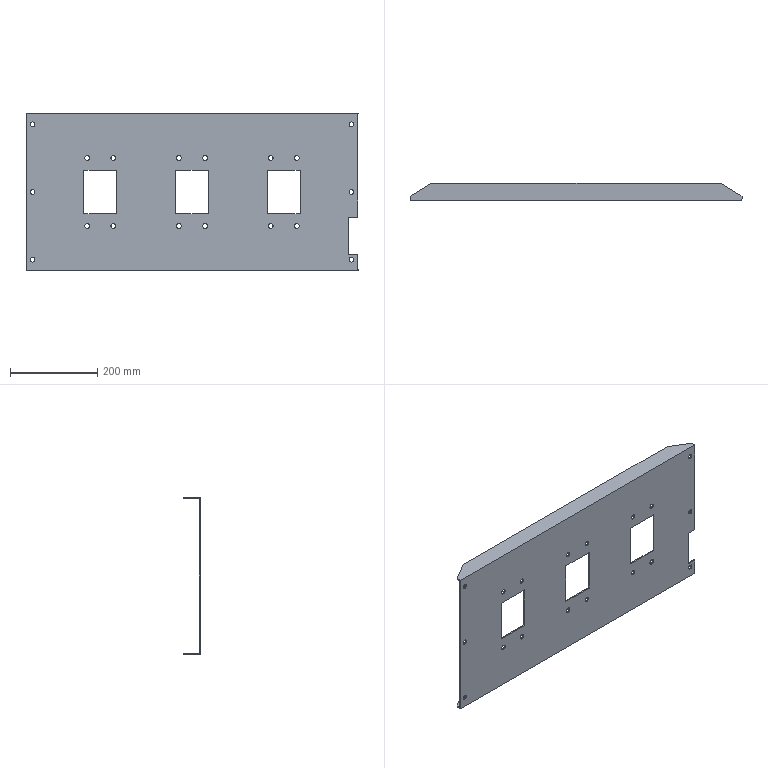Part | SolidWorks | features BaseBody 1 | 1 solid | 66 faces | box 760 x 40 x 360 mm | volume 902338 mm3 | cylinder 36 | plane 30 | commonest cylinder face diameters 11.1 x24 10.6 x12